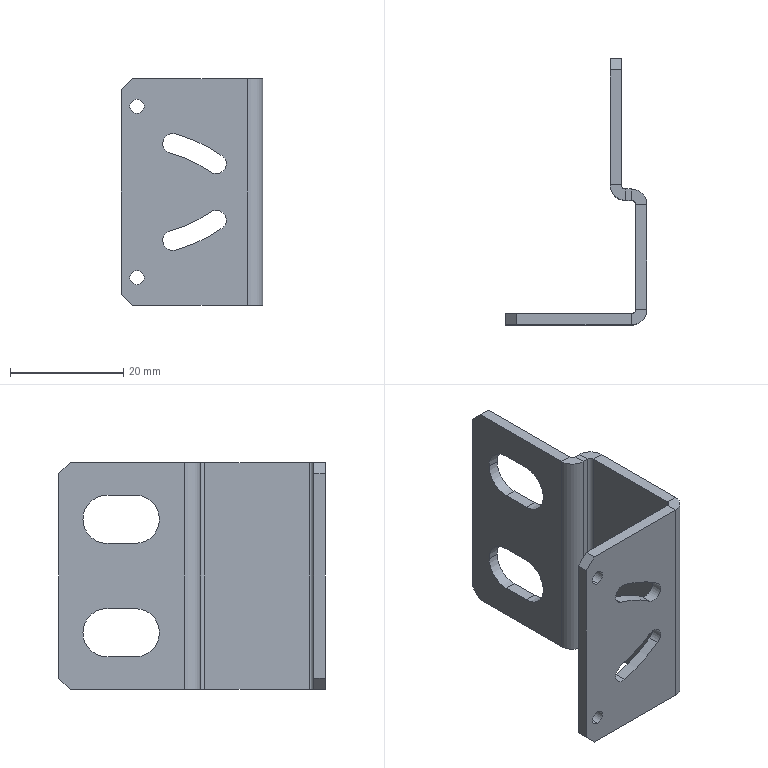Part | STEP file | 09-31 micro switch seat (Default) | 1 solid | 58 faces | box 25 x 47 x 40 mm | volume 5190 mm3 | plane 32 | cylinder 26 | commonest cylinder face diameters 3.5 x6 8.5 x6 2.5 x4 1.473 x3 5.473 x3 45.446 x2